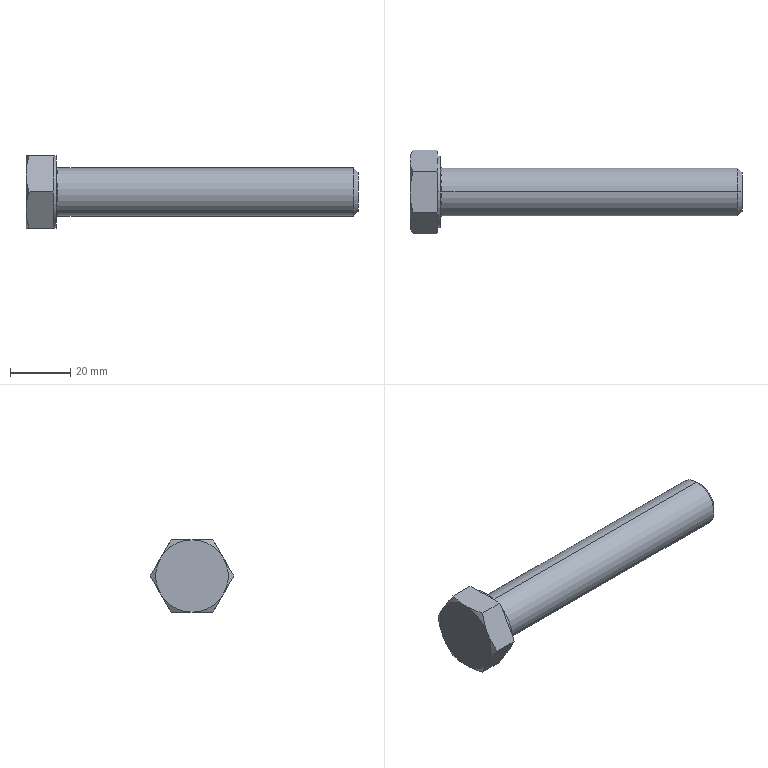Part | STEP file | 1 solid | 35 faces | box 110 x 27.713 x 24 mm | volume 24987 mm3 | plane 15 | cone 14 | cylinder 4 | spline 2 | commonest cylinder face diameters 16 x2 24 x2